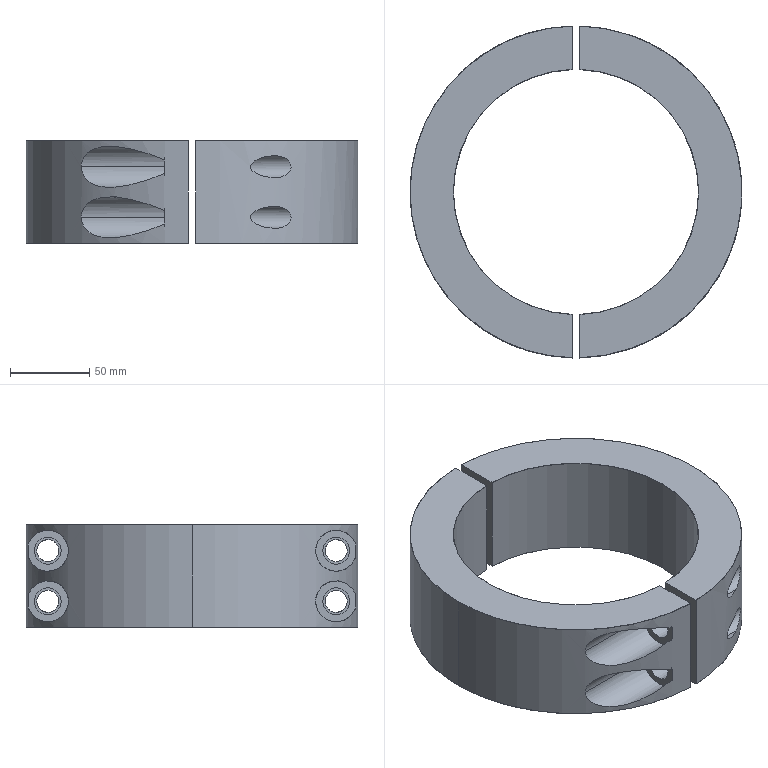Part | SolidWorks | features ICE 4, MirrorPattern 3, Chamfer 1, Extrusion 1, HoleWzd 1 | 2 solids | 52 faces | box 210 x 209.94 x 65 mm | volume 894732 mm3 | cylinder 28 | cone 12 | plane 12 | commonest cylinder face diameters 14 x8 17 x8 26 x6 155 x3 210 x3